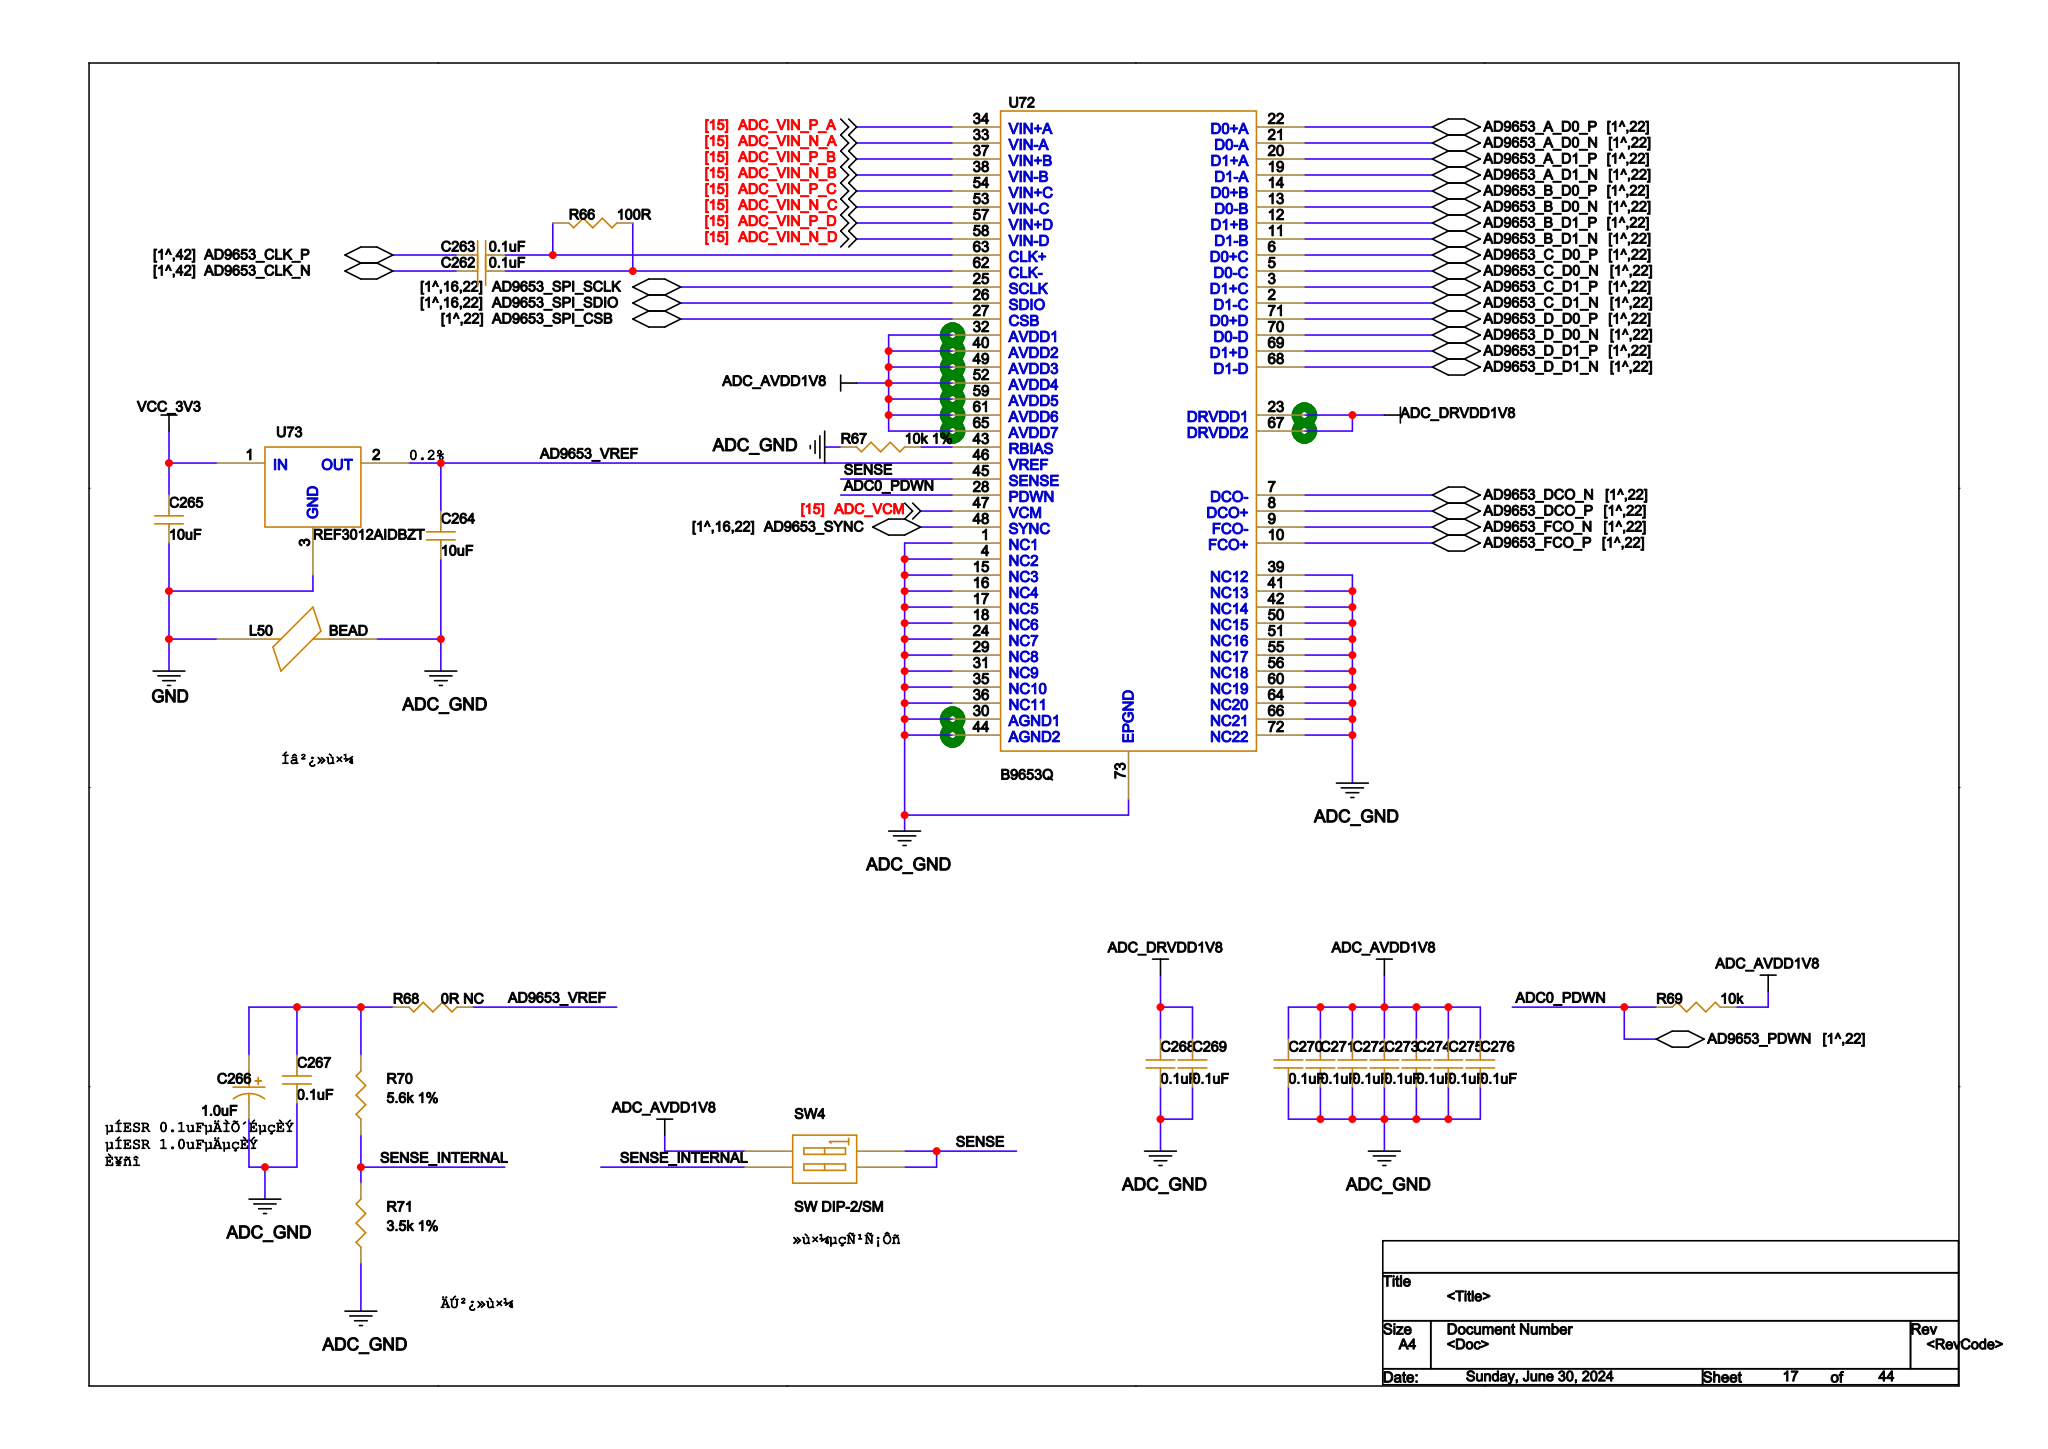Circuit board | Cadence Allegro | 1034 parts | 912 nets | one sheet of the schematic
Parts on this sheet (reference | value | footprint):
C262 | 0.1uF | C0402
C263 | 0.1uF | C0402
C264 | 10uF | C0402
C265 | 10uF | C0402
C266 | 1.0uF | C0402
C267 | 0.1uF | C0402
C268 | 0.1uF | C0402
C269 | 0.1uF | C0402
C270 | 0.1uF | C0402
C271 | 0.1uF | C0402
C272 | 0.1uF | C0402
C273 | 0.1uF | C0402
C274 | 0.1uF | C0402
C275 | 0.1uF | C0402
C276 | 0.1uF | C0402
L50 | BEAD | PZ2012
R66 | 100R | R0402
R67 | 10k 1% | R0402
R68 | 0R NC | R0402
R69 | 10k | R0402
R70 | 5.6k 1% | R0402
R71 | 3.5k 1% | R0402
SW4 | SW DIP-2/SM | SW_2_SOP
U72 | B9653Q | B9653Q_CQFP72
U73 | REF3012AIDBZT | REF3012_SOT23
Nets of these parts (net: part-pin ...):
GND: C265-1 L50-1 U73-3
VCC_3V3: C265-2 U73-1
N186588: C263-2
N186604: C262-2
ADC_GND: C264-1 C266-2 C267-1 C268-1 C269-1 C270-1 C271-1 C272-1 C273-1 C274-1 C275-1 C276-1 L50-2 R67-2 R71-1 U72-1 U72-4 U72-15 U72-16 U72-17 U72-18 U72-24 U72-29 U72-30 U72-31 U72-35 U72-36 U72-39 U72-41 U72-42 U72-44 U72-50 U72-51 U72-55 U72-56 U72-60 U72-64 U72-66 U72-72 U72-73
ADC_AVDD1V8: C270-2 C271-2 C272-2 C273-2 C274-2 C275-2 C276-2 R69-2 SW4-1 U72-32 U72-40 U72-49 U72-52 U72-59 U72-61 U72-65
ADC_DRVDD1V8: C268-2 C269-2 U72-67
N111291_D4: C263-1 R66-2 U72-63
N111295_D4: C262-1 R66-1 U72-62
N187560: R69-1 U72-28
N110707_D4: R67-1 U72-43
SENSE_D4: SW4-3 SW4-4 U72-45
AD9653_VREF_D4: C264-2 R68-1 U73-2 U72-46
N14127011_D4: C266-1 C267-2 R68-2 R70-2
SENSE_INTERNAL_D4: R70-1 R71-2 SW4-2